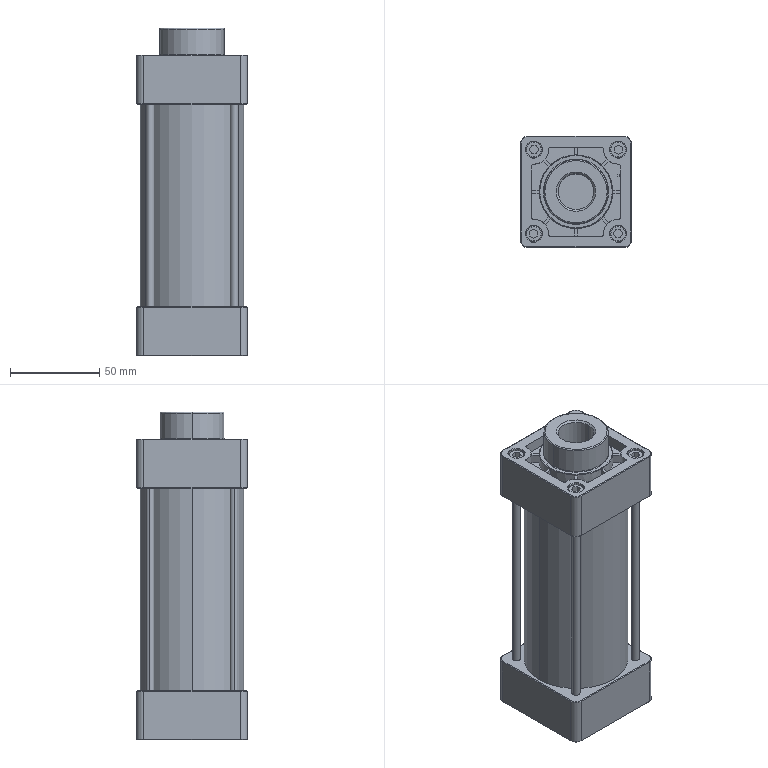Part | STEP file | 2 solids | 348 faces | box 62 x 62 x 183 mm | volume 287709 mm3 | plane 162 | cylinder 112 | cone 44 | torus 26 | spline 4 | commonest cylinder face diameters 12.301 x30 8.6 x16 9 x16 2 x10 4.5 x8 8 x8